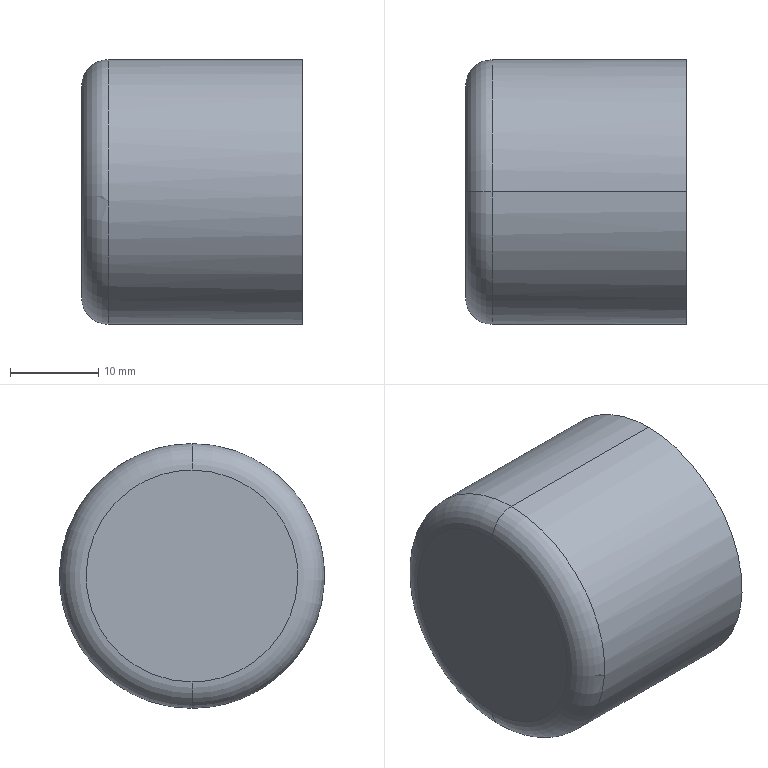Part | SolidWorks | features BaseBody 1 | 1 solid | 11 faces | box 25 x 30 x 30 mm | volume 13143 mm3 | cylinder 4 | plane 3 | cone 2 | torus 2 | commonest cylinder face diameters 18 x2 30 x2
STEP:
#1=CARTESIAN_POINT('',(7.,0.,6.));
#2=VERTEX_POINT('',#1);
#3=CARTESIAN_POINT('',(7.,0.,-6.));
#4=VERTEX_POINT('',#3);
#5=CARTESIAN_POINT('',(7.,0.,6.));
#6=CARTESIAN_POINT('',(7.,-0.7879,6.));
#7=CARTESIAN_POINT('',(7.,-1.568,5.845));
#8=CARTESIAN_POINT('',(7.,-3.024,5.242));
#9=CARTESIAN_POINT('',(7.,-3.685,4.8));
#10=CARTESIAN_POINT('',(7.,-4.8,3.685));
#11=CARTESIAN_POINT('',(7.,-5.242,3.024));
#12=CARTESIAN_POINT('',(7.,-5.845,1.568));
#13=CARTESIAN_POINT('',(7.,-6.,0.7879));
#14=CARTESIAN_POINT('',(7.,-6.,-0.7879));
#15=CARTESIAN_POINT('',(7.,-5.845,-1.568));
#16=CARTESIAN_POINT('',(7.,-5.242,-3.024));
#17=CARTESIAN_POINT('',(7.,-4.8,-3.685));
#18=CARTESIAN_POINT('',(7.,-3.685,-4.8));
#19=CARTESIAN_POINT('',(7.,-3.024,-5.242));
#20=CARTESIAN_POINT('',(7.,-1.568,-5.845));
#21=CARTESIAN_POINT('',(7.,-0.7879,-6.));
#22=CARTESIAN_POINT('',(7.,0.,-6.));
#23=B_SPLINE_CURVE_WITH_KNOTS('',3,(#5,#6,#7,#8,#9,#10,#11,#12,#13,#14,#15,#16,#17,#18,#19,#20,#21,#22),.UNSPECIFIED.,.F.,.F.,(4,2,2,2,2,2,2,2,4),(3.142,3.534,3.927,4.32,4.712,5.105,5.498,5.89,6.283),.UNSPECIFIED.);
#24=EDGE_CURVE('',#2,#4,#23,.T.);
#25=ORIENTED_EDGE('',*,*,#24,.F.);
#26=CARTESIAN_POINT('',(10.,0.,9.));
#27=VERTEX_POINT('',#26);
#28=CARTESIAN_POINT('',(10.,0.,9.));
#29=DIRECTION('',(0.7071,0.,0.7071));
#30=VECTOR('',#29,1000.);
#31=LINE('',#28,#30);
#32=EDGE_CURVE('',#2,#27,#31,.T.);
#33=ORIENTED_EDGE('',*,*,#32,.T.);
#34=CARTESIAN_POINT('',(10.,0.,-9.));
#35=VERTEX_POINT('',#34);
#36=CARTESIAN_POINT('',(10.,0.,9.));
#37=CARTESIAN_POINT('',(10.,-1.178,9.));
#38=CARTESIAN_POINT('',(10.,-2.356,8.766));
#39=CARTESIAN_POINT('',(10.,-4.533,7.864));
#40=CARTESIAN_POINT('',(10.,-5.531,7.197));
#41=CARTESIAN_POINT('',(10.,-7.197,5.531));
#42=CARTESIAN_POINT('',(10.,-7.864,4.533));
#43=CARTESIAN_POINT('',(10.,-8.766,2.356));
#44=CARTESIAN_POINT('',(10.,-9.,1.178));
#45=CARTESIAN_POINT('',(10.,-9.,-1.178));
#46=CARTESIAN_POINT('',(10.,-8.766,-2.356));
#47=CARTESIAN_POINT('',(10.,-7.864,-4.533));
#48=CARTESIAN_POINT('',(10.,-7.197,-5.531));
#49=CARTESIAN_POINT('',(10.,-5.531,-7.197));
#50=CARTESIAN_POINT('',(10.,-4.533,-7.864));
#51=CARTESIAN_POINT('',(10.,-2.356,-8.766));
#52=CARTESIAN_POINT('',(10.,-1.178,-9.));
#53=CARTESIAN_POINT('',(10.,0.,-9.));
#54=B_SPLINE_CURVE_WITH_KNOTS('',3,(#36,#37,#38,#39,#40,#41,#42,#43,#44,#45,#46,#47,#48,#49,#50,#51,#52,#53),.UNSPECIFIED.,.F.,.F.,(4,2,2,2,2,2,2,2,4),(3.142,3.534,3.927,4.32,4.712,5.105,5.498,5.89,6.283),.UNSPECIFIED.);
#55=EDGE_CURVE('',#27,#35,#54,.T.);
#56=ORIENTED_EDGE('',*,*,#55,.T.);
#57=CARTESIAN_POINT('',(10.,0.,-9.));
#58=DIRECTION('',(0.7071,0.,-0.7071));
#59=VECTOR('',#58,1000.);
#60=LINE('',#57,#59);
#61=EDGE_CURVE('',#4,#35,#60,.T.);
#62=ORIENTED_EDGE('',*,*,#61,.F.);
#63=EDGE_LOOP('',(#25,#33,#56,#62));
#64=FACE_OUTER_BOUND('',#63,.T.);
#65=CARTESIAN_POINT('',(10.,0.,0.));
#66=DIRECTION('',(1.,0.,0.));
#67=DIRECTION('',(0.,0.,-1.));
#68=AXIS2_PLACEMENT_3D('',#65,#66,#67);
#69=CONICAL_SURFACE('',#68,9.,0.7854);
#70=ADVANCED_FACE('',(#64),#69,.F.);
#71=ORIENTED_EDGE('',*,*,#55,.F.);
#72=CARTESIAN_POINT('',(25.,0.,9.));
#73=VERTEX_POINT('',#72);
#74=CARTESIAN_POINT('',(35.,0.,9.));
#75=DIRECTION('',(1.,0.,0.));
#76=VECTOR('',#75,1000.);
#77=LINE('',#74,#76);
#78=EDGE_CURVE('',#27,#73,#77,.T.);
#79=ORIENTED_EDGE('',*,*,#78,.T.);
#80=CARTESIAN_POINT('',(25.,0.,-9.));
#81=VERTEX_POINT('',#80);
#82=CARTESIAN_POINT('',(25.,0.,9.));
#83=CARTESIAN_POINT('',(25.,-1.178,9.));
#84=CARTESIAN_POINT('',(25.,-2.356,8.766));
#85=CARTESIAN_POINT('',(25.,-4.533,7.864));
#86=CARTESIAN_POINT('',(25.,-5.531,7.197));
#87=CARTESIAN_POINT('',(25.,-7.197,5.531));
#88=CARTESIAN_POINT('',(25.,-7.864,4.533));
#89=CARTESIAN_POINT('',(25.,-8.766,2.356));
#90=CARTESIAN_POINT('',(25.,-9.,1.178));
#91=CARTESIAN_POINT('',(25.,-9.,-1.178));
#92=CARTESIAN_POINT('',(25.,-8.766,-2.356));
#93=CARTESIAN_POINT('',(25.,-7.864,-4.533));
#94=CARTESIAN_POINT('',(25.,-7.197,-5.531));
#95=CARTESIAN_POINT('',(25.,-5.531,-7.197));
#96=CARTESIAN_POINT('',(25.,-4.533,-7.864));
#97=CARTESIAN_POINT('',(25.,-2.356,-8.766));
#98=CARTESIAN_POINT('',(25.,-1.178,-9.));
#99=CARTESIAN_POINT('',(25.,0.,-9.));
#100=B_SPLINE_CURVE_WITH_KNOTS('',3,(#82,#83,#84,#85,#86,#87,#88,#89,#90,#91,#92,#93,#94,#95,#96,#97,#98,#99),.UNSPECIFIED.,.F.,.F.,(4,2,2,2,2,2,2,2,4),(3.142,3.534,3.927,4.32,4.712,5.105,5.498,5.89,6.283),.UNSPECIFIED.);
#101=EDGE_CURVE('',#73,#81,#100,.T.);
#102=ORIENTED_EDGE('',*,*,#101,.T.);
#103=CARTESIAN_POINT('',(35.,0.,-9.));
#104=DIRECTION('',(1.,0.,0.));
#105=VECTOR('',#104,1000.);
#106=LINE('',#103,#105);
#107=EDGE_CURVE('',#35,#81,#106,.T.);
#108=ORIENTED_EDGE('',*,*,#107,.F.);
#109=EDGE_LOOP('',(#71,#79,#102,#108));
#110=FACE_OUTER_BOUND('',#109,.T.);
#111=CARTESIAN_POINT('',(35.,0.,0.));
#112=DIRECTION('',(1.,0.,0.));
#113=DIRECTION('',(0.,0.,-1.));
#114=AXIS2_PLACEMENT_3D('',#111,#112,#113);
#115=CYLINDRICAL_SURFACE('',#114,9.);
#116=ADVANCED_FACE('',(#110),#115,.F.);
#117=CARTESIAN_POINT('',(3.,0.,-15.));
#118=VERTEX_POINT('',#117);
#119=CARTESIAN_POINT('',(3.,0.,15.));
#120=VERTEX_POINT('',#119);
#121=CARTESIAN_POINT('',(3.,0.,-15.));
#122=CARTESIAN_POINT('',(3.,1.963,-15.));
#123=CARTESIAN_POINT('',(3.,3.926,-14.61));
#124=CARTESIAN_POINT('',(3.,7.554,-13.107));
#125=CARTESIAN_POINT('',(3.,9.218,-11.995));
#126=CARTESIAN_POINT('',(3.,11.995,-9.218));
#127=CARTESIAN_POINT('',(3.,13.107,-7.554));
#128=CARTESIAN_POINT('',(3.,14.61,-3.926));
#129=CARTESIAN_POINT('',(3.,15.,-1.963));
#130=CARTESIAN_POINT('',(3.,15.,1.963));
#131=CARTESIAN_POINT('',(3.,14.61,3.926));
#132=CARTESIAN_POINT('',(3.,13.107,7.554));
#133=CARTESIAN_POINT('',(3.,11.995,9.218));
#134=CARTESIAN_POINT('',(3.,9.218,11.995));
#135=CARTESIAN_POINT('',(3.,7.554,13.107));
#136=CARTESIAN_POINT('',(3.,3.926,14.61));
#137=CARTESIAN_POINT('',(3.,1.963,15.));
#138=CARTESIAN_POINT('',(3.,0.,15.));
#139=B_SPLINE_CURVE_WITH_KNOTS('',3,(#121,#122,#123,#124,#125,#126,#127,#128,#129,#130,#131,#132,#133,#134,#135,#136,#137,#138),.UNSPECIFIED.,.F.,.F.,(4,2,2,2,2,2,2,2,4),(0.,0.3927,0.7854,1.178,1.571,1.963,2.356,2.749,3.142),.UNSPECIFIED.);
#140=EDGE_CURVE('',#118,#120,#139,.T.);
#141=ORIENTED_EDGE('',*,*,#140,.T.);
#142=CARTESIAN_POINT('',(25.,0.,15.));
#143=VERTEX_POINT('',#142);
#144=CARTESIAN_POINT('',(35.,0.,15.));
#145=DIRECTION('',(1.,0.,0.));
#146=VECTOR('',#145,1000.);
#147=LINE('',#144,#146);
#148=EDGE_CURVE('',#120,#143,#147,.T.);
#149=ORIENTED_EDGE('',*,*,#148,.T.);
#150=CARTESIAN_POINT('',(25.,0.,-15.));
#151=VERTEX_POINT('',#150);
#152=CARTESIAN_POINT('',(25.,0.,-15.));
#153=CARTESIAN_POINT('',(25.,0.9849,-15.));
#154=CARTESIAN_POINT('',(25.,1.96,-14.904));
#155=CARTESIAN_POINT('',(25.,3.892,-14.52));
#156=CARTESIAN_POINT('',(25.,4.83,-14.235));
#157=CARTESIAN_POINT('',(25.,6.65,-13.481));
#158=CARTESIAN_POINT('',(25.,7.515,-13.019));
#159=CARTESIAN_POINT('',(25.,9.152,-11.925));
#160=CARTESIAN_POINT('',(25.,9.91,-11.303));
#161=CARTESIAN_POINT('',(25.,11.303,-9.91));
#162=CARTESIAN_POINT('',(25.,11.925,-9.152));
#163=CARTESIAN_POINT('',(25.,13.019,-7.515));
#164=CARTESIAN_POINT('',(25.,13.481,-6.65));
#165=CARTESIAN_POINT('',(25.,14.235,-4.83));
#166=CARTESIAN_POINT('',(25.,14.52,-3.892));
#167=CARTESIAN_POINT('',(25.,14.904,-1.96));
#168=CARTESIAN_POINT('',(25.,15.,-0.9849));
#169=CARTESIAN_POINT('',(25.,15.,0.9849));
#170=CARTESIAN_POINT('',(25.,14.904,1.96));
#171=CARTESIAN_POINT('',(25.,14.52,3.892));
#172=CARTESIAN_POINT('',(25.,14.235,4.83));
#173=CARTESIAN_POINT('',(25.,13.481,6.65));
#174=CARTESIAN_POINT('',(25.,13.019,7.515));
#175=CARTESIAN_POINT('',(25.,11.925,9.152));
#176=CARTESIAN_POINT('',(25.,11.303,9.91));
#177=CARTESIAN_POINT('',(25.,9.91,11.303));
#178=CARTESIAN_POINT('',(25.,9.152,11.925));
#179=CARTESIAN_POINT('',(25.,7.515,13.019));
#180=CARTESIAN_POINT('',(25.,6.65,13.481));
#181=CARTESIAN_POINT('',(25.,4.83,14.235));
#182=CARTESIAN_POINT('',(25.,3.892,14.52));
#183=CARTESIAN_POINT('',(25.,1.96,14.904));
#184=CARTESIAN_POINT('',(25.,0.9849,15.));
#185=CARTESIAN_POINT('',(25.,0.,15.));
#186=B_SPLINE_CURVE_WITH_KNOTS('',3,(#152,#153,#154,#155,#156,#157,#158,#159,#160,#161,#162,#163,#164,#165,#166,#167,#168,#169,#170,#171,#172,#173,#174,#175,#176,#177,#178,#179,#180,#181,#182,#183,#184,#185),.UNSPECIFIED.,.F.,.F.,(4,2,2,2,2,2,2,2,2,2,2,2,2,2,2,2,4),(0.,0.1963,0.3927,0.589,0.7854,0.9817,1.178,1.374,1.571,1.767,1.963,2.16,2.356,2.553,2.749,2.945,3.142),.UNSPECIFIED.);
#187=EDGE_CURVE('',#151,#143,#186,.T.);
#188=ORIENTED_EDGE('',*,*,#187,.F.);
#189=CARTESIAN_POINT('',(35.,0.,-15.));
#190=DIRECTION('',(1.,0.,0.));
#191=VECTOR('',#190,1000.);
#192=LINE('',#189,#191);
#193=EDGE_CURVE('',#118,#151,#192,.T.);
#194=ORIENTED_EDGE('',*,*,#193,.F.);
#195=EDGE_LOOP('',(#141,#149,#188,#194));
#196=FACE_OUTER_BOUND('',#195,.T.);
#197=CARTESIAN_POINT('',(35.,0.,0.));
#198=DIRECTION('',(1.,0.,0.));
#199=DIRECTION('',(0.,0.,-1.));
#200=AXIS2_PLACEMENT_3D('',#197,#198,#199);
#201=CYLINDRICAL_SURFACE('',#200,15.);
#202=ADVANCED_FACE('',(#196),#201,.T.);
#203=CARTESIAN_POINT('',(0.,0.,-12.));
#204=VERTEX_POINT('',#203);
#205=CARTESIAN_POINT('',(0.,0.,12.));
#206=VERTEX_POINT('',#205);
#207=CARTESIAN_POINT('',(0.,0.,-12.));
#208=CARTESIAN_POINT('',(0.,1.571,-12.));
#209=CARTESIAN_POINT('',(0.,3.141,-11.688));
#210=CARTESIAN_POINT('',(0.,6.043,-10.485));
#211=CARTESIAN_POINT('',(0.,7.375,-9.596));
#212=CARTESIAN_POINT('',(0.,9.596,-7.375));
#213=CARTESIAN_POINT('',(0.,10.485,-6.043));
#214=CARTESIAN_POINT('',(0.,11.688,-3.141));
#215=CARTESIAN_POINT('',(0.,12.,-1.571));
#216=CARTESIAN_POINT('',(0.,12.,1.571));
#217=CARTESIAN_POINT('',(0.,11.688,3.141));
#218=CARTESIAN_POINT('',(0.,10.485,6.043));
#219=CARTESIAN_POINT('',(0.,9.596,7.375));
#220=CARTESIAN_POINT('',(0.,7.375,9.596));
#221=CARTESIAN_POINT('',(0.,6.043,10.485));
#222=CARTESIAN_POINT('',(0.,3.141,11.688));
#223=CARTESIAN_POINT('',(0.,1.571,12.));
#224=CARTESIAN_POINT('',(0.,0.,12.));
#225=B_SPLINE_CURVE_WITH_KNOTS('',3,(#207,#208,#209,#210,#211,#212,#213,#214,#215,#216,#217,#218,#219,#220,#221,#222,#223,#224),.UNSPECIFIED.,.F.,.F.,(4,2,2,2,2,2,2,2,4),(0.,0.3927,0.7854,1.178,1.571,1.963,2.356,2.749,3.142),.UNSPECIFIED.);
#226=EDGE_CURVE('',#204,#206,#225,.T.);
#227=ORIENTED_EDGE('',*,*,#226,.T.);
#228=CARTESIAN_POINT('',(3.,0.,12.));
#229=DIRECTION('',(0.,1.,0.));
#230=DIRECTION('',(0.,0.,1.));
#231=AXIS2_PLACEMENT_3D('',#228,#229,#230);
#232=CIRCLE('',#231,3.);
#233=EDGE_CURVE('',#206,#120,#232,.T.);
#234=ORIENTED_EDGE('',*,*,#233,.T.);
#235=ORIENTED_EDGE('',*,*,#140,.F.);
#236=CARTESIAN_POINT('',(3.,0.,-12.));
#237=DIRECTION('',(0.,-1.,0.));
#238=DIRECTION('',(0.,0.,-1.));
#239=AXIS2_PLACEMENT_3D('',#236,#237,#238);
#240=CIRCLE('',#239,3.);
#241=EDGE_CURVE('',#204,#118,#240,.T.);
#242=ORIENTED_EDGE('',*,*,#241,.F.);
#243=EDGE_LOOP('',(#227,#234,#235,#242));
#244=FACE_OUTER_BOUND('',#243,.T.);
#245=CARTESIAN_POINT('',(3.,0.,0.));
#246=DIRECTION('',(1.,0.,0.));
#247=DIRECTION('',(0.,0.,-1.));
#248=AXIS2_PLACEMENT_3D('',#245,#246,#247);
#249=TOROIDAL_SURFACE('',#248,12.,3.);
#250=ADVANCED_FACE('',(#244),#249,.T.);
#251=ORIENTED_EDGE('',*,*,#226,.F.);
#252=CARTESIAN_POINT('',(0.,0.,12.));
#253=CARTESIAN_POINT('',(0.,-1.571,12.));
#254=CARTESIAN_POINT('',(0.,-3.141,11.688));
#255=CARTESIAN_POINT('',(0.,-6.043,10.485));
#256=CARTESIAN_POINT('',(0.,-7.375,9.596));
#257=CARTESIAN_POINT('',(0.,-9.596,7.375));
#258=CARTESIAN_POINT('',(0.,-10.485,6.043));
#259=CARTESIAN_POINT('',(0.,-11.688,3.141));
#260=CARTESIAN_POINT('',(0.,-12.,1.571));
#261=CARTESIAN_POINT('',(0.,-12.,-1.571));
#262=CARTESIAN_POINT('',(0.,-11.688,-3.141));
#263=CARTESIAN_POINT('',(0.,-10.485,-6.043));
#264=CARTESIAN_POINT('',(0.,-9.596,-7.375));
#265=CARTESIAN_POINT('',(0.,-7.375,-9.596));
#266=CARTESIAN_POINT('',(0.,-6.043,-10.485));
#267=CARTESIAN_POINT('',(0.,-3.141,-11.688));
#268=CARTESIAN_POINT('',(0.,-1.571,-12.));
#269=CARTESIAN_POINT('',(0.,0.,-12.));
#270=B_SPLINE_CURVE_WITH_KNOTS('',3,(#252,#253,#254,#255,#256,#257,#258,#259,#260,#261,#262,#263,#264,#265,#266,#267,#268,#269),.UNSPECIFIED.,.F.,.F.,(4,2,2,2,2,2,2,2,4),(3.142,3.534,3.927,4.32,4.712,5.105,5.498,5.89,6.283),.UNSPECIFIED.);
#271=EDGE_CURVE('',#206,#204,#270,.T.);
#272=ORIENTED_EDGE('',*,*,#271,.F.);
#273=EDGE_LOOP('',(#251,#272));
#274=FACE_OUTER_BOUND('',#273,.T.);
#275=CARTESIAN_POINT('',(0.,0.,0.));
#276=DIRECTION('',(1.,0.,0.));
#277=DIRECTION('',(0.,0.,-1.));
#278=AXIS2_PLACEMENT_3D('',#275,#276,#277);
#279=PLANE('',#278);
#280=ADVANCED_FACE('',(#274),#279,.F.);
#281=ORIENTED_EDGE('',*,*,#233,.F.);
#282=ORIENTED_EDGE('',*,*,#271,.T.);
#283=ORIENTED_EDGE('',*,*,#241,.T.);
#284=CARTESIAN_POINT('',(3.,0.,15.));
#285=CARTESIAN_POINT('',(3.,-1.963,15.));
#286=CARTESIAN_POINT('',(3.,-3.926,14.61));
#287=CARTESIAN_POINT('',(3.,-7.554,13.107));
#288=CARTESIAN_POINT('',(3.,-9.218,11.995));
#289=CARTESIAN_POINT('',(3.,-11.995,9.218));
#290=CARTESIAN_POINT('',(3.,-13.107,7.554));
#291=CARTESIAN_POINT('',(3.,-14.61,3.926));
#292=CARTESIAN_POINT('',(3.,-15.,1.963));
#293=CARTESIAN_POINT('',(3.,-15.,-1.963));
#294=CARTESIAN_POINT('',(3.,-14.61,-3.926));
#295=CARTESIAN_POINT('',(3.,-13.107,-7.554));
#296=CARTESIAN_POINT('',(3.,-11.995,-9.218));
#297=CARTESIAN_POINT('',(3.,-9.218,-11.995));
#298=CARTESIAN_POINT('',(3.,-7.554,-13.107));
#299=CARTESIAN_POINT('',(3.,-3.926,-14.61));
#300=CARTESIAN_POINT('',(3.,-1.963,-15.));
#301=CARTESIAN_POINT('',(3.,0.,-15.));
#302=B_SPLINE_CURVE_WITH_KNOTS('',3,(#284,#285,#286,#287,#288,#289,#290,#291,#292,#293,#294,#295,#296,#297,#298,#299,#300,#301),.UNSPECIFIED.,.F.,.F.,(4,2,2,2,2,2,2,2,4),(3.142,3.534,3.927,4.32,4.712,5.105,5.498,5.89,6.283),.UNSPECIFIED.);
#303=EDGE_CURVE('',#120,#118,#302,.T.);
#304=ORIENTED_EDGE('',*,*,#303,.F.);
#305=EDGE_LOOP('',(#281,#282,#283,#304));
#306=FACE_OUTER_BOUND('',#305,.T.);
#307=CARTESIAN_POINT('',(3.,0.,0.));
#308=DIRECTION('',(1.,0.,0.));
#309=DIRECTION('',(0.,0.,-1.));
#310=AXIS2_PLACEMENT_3D('',#307,#308,#309);
#311=TOROIDAL_SURFACE('',#310,12.,3.);
#312=ADVANCED_FACE('',(#306),#311,.T.);
#313=ORIENTED_EDGE('',*,*,#148,.F.);
#314=ORIENTED_EDGE('',*,*,#303,.T.);
#315=ORIENTED_EDGE('',*,*,#193,.T.);
#316=CARTESIAN_POINT('',(25.,0.,15.));
#317=CARTESIAN_POINT('',(25.,-0.9849,15.));
#318=CARTESIAN_POINT('',(25.,-1.96,14.904));
#319=CARTESIAN_POINT('',(25.,-3.892,14.52));
#320=CARTESIAN_POINT('',(25.,-4.83,14.235));
#321=CARTESIAN_POINT('',(25.,-6.65,13.481));
#322=CARTESIAN_POINT('',(25.,-7.515,13.019));
#323=CARTESIAN_POINT('',(25.,-9.152,11.925));
#324=CARTESIAN_POINT('',(25.,-9.91,11.303));
#325=CARTESIAN_POINT('',(25.,-11.303,9.91));
#326=CARTESIAN_POINT('',(25.,-11.925,9.152));
#327=CARTESIAN_POINT('',(25.,-13.019,7.515));
#328=CARTESIAN_POINT('',(25.,-13.481,6.65));
#329=CARTESIAN_POINT('',(25.,-14.235,4.83));
#330=CARTESIAN_POINT('',(25.,-14.52,3.892));
#331=CARTESIAN_POINT('',(25.,-14.904,1.96));
#332=CARTESIAN_POINT('',(25.,-15.,0.9849));
#333=CARTESIAN_POINT('',(25.,-15.,-0.9849));
#334=CARTESIAN_POINT('',(25.,-14.904,-1.96));
#335=CARTESIAN_POINT('',(25.,-14.52,-3.892));
#336=CARTESIAN_POINT('',(25.,-14.235,-4.83));
#337=CARTESIAN_POINT('',(25.,-13.481,-6.65));
#338=CARTESIAN_POINT('',(25.,-13.019,-7.515));
#339=CARTESIAN_POINT('',(25.,-11.925,-9.152));
#340=CARTESIAN_POINT('',(25.,-11.303,-9.91));
#341=CARTESIAN_POINT('',(25.,-9.91,-11.303));
#342=CARTESIAN_POINT('',(25.,-9.152,-11.925));
#343=CARTESIAN_POINT('',(25.,-7.515,-13.019));
#344=CARTESIAN_POINT('',(25.,-6.65,-13.481));
#345=CARTESIAN_POINT('',(25.,-4.83,-14.235));
#346=CARTESIAN_POINT('',(25.,-3.892,-14.52));
#347=CARTESIAN_POINT('',(25.,-1.96,-14.904));
#348=CARTESIAN_POINT('',(25.,-0.9849,-15.));
#349=CARTESIAN_POINT('',(25.,0.,-15.));
#350=B_SPLINE_CURVE_WITH_KNOTS('',3,(#316,#317,#318,#319,#320,#321,#322,#323,#324,#325,#326,#327,#328,#329,#330,#331,#332,#333,#334,#335,#336,#337,#338,#339,#340,#341,#342,#343,#344,#345,#346,#347,#348,#349),.UNSPECIFIED.,.F.,.F.,(4,2,2,2,2,2,2,2,2,2,2,2,2,2,2,2,4),(3.142,3.338,3.534,3.731,3.927,4.123,4.32,4.516,4.712,4.909,5.105,5.301,5.498,5.694,5.89,6.087,6.283),.UNSPECIFIED.);
#351=EDGE_CURVE('',#143,#151,#350,.T.);
#352=ORIENTED_EDGE('',*,*,#351,.F.);
#353=EDGE_LOOP('',(#313,#314,#315,#352));
#354=FACE_OUTER_BOUND('',#353,.T.);
#355=CARTESIAN_POINT('',(35.,0.,0.));
#356=DIRECTION('',(1.,0.,0.));
#357=DIRECTION('',(0.,0.,-1.));
#358=AXIS2_PLACEMENT_3D('',#355,#356,#357);
#359=CYLINDRICAL_SURFACE('',#358,15.);
#360=ADVANCED_FACE('',(#354),#359,.T.);
#361=CARTESIAN_POINT('',(25.,0.,-9.));
#362=CARTESIAN_POINT('',(25.,1.178,-9.));
#363=CARTESIAN_POINT('',(25.,2.356,-8.766));
#364=CARTESIAN_POINT('',(25.,4.533,-7.864));
#365=CARTESIAN_POINT('',(25.,5.531,-7.197));
#366=CARTESIAN_POINT('',(25.,7.197,-5.531));
#367=CARTESIAN_POINT('',(25.,7.864,-4.533));
#368=CARTESIAN_POINT('',(25.,8.766,-2.356));
#369=CARTESIAN_POINT('',(25.,9.,-1.178));
#370=CARTESIAN_POINT('',(25.,9.,1.178));
#371=CARTESIAN_POINT('',(25.,8.766,2.356));
#372=CARTESIAN_POINT('',(25.,7.864,4.533));
#373=CARTESIAN_POINT('',(25.,7.197,5.531));
#374=CARTESIAN_POINT('',(25.,5.531,7.197));
#375=CARTESIAN_POINT('',(25.,4.533,7.864));
#376=CARTESIAN_POINT('',(25.,2.356,8.766));
#377=CARTESIAN_POINT('',(25.,1.178,9.));
#378=CARTESIAN_POINT('',(25.,0.,9.));
#379=B_SPLINE_CURVE_WITH_KNOTS('',3,(#361,#362,#363,#364,#365,#366,#367,#368,#369,#370,#371,#372,#373,#374,#375,#376,#377,#378),.UNSPECIFIED.,.F.,.F.,(4,2,2,2,2,2,2,2,4),(0.,0.3927,0.7854,1.178,1.571,1.963,2.356,2.749,3.142),.UNSPECIFIED.);
#380=EDGE_CURVE('',#81,#73,#379,.T.);
#381=ORIENTED_EDGE('',*,*,#380,.F.);
#382=ORIENTED_EDGE('',*,*,#101,.F.);
#383=EDGE_LOOP('',(#381,#382));
#384=FACE_BOUND('',#383,.T.);
#385=ORIENTED_EDGE('',*,*,#187,.T.);
#386=ORIENTED_EDGE('',*,*,#351,.T.);
#387=EDGE_LOOP('',(#385,#386));
#388=FACE_OUTER_BOUND('',#387,.T.);
#389=CARTESIAN_POINT('',(25.,15.,0.));
#390=DIRECTION('',(-1.,0.,0.));
#391=DIRECTION('',(0.,0.,1.));
#392=AXIS2_PLACEMENT_3D('',#389,#390,#391);
#393=PLANE('',#392);
#394=ADVANCED_FACE('',(#384,#388),#393,.F.);
#395=ORIENTED_EDGE('',*,*,#78,.F.);
#396=CARTESIAN_POINT('',(10.,0.,-9.));
#397=CARTESIAN_POINT('',(10.,1.178,-9.));
#398=CARTESIAN_POINT('',(10.,2.356,-8.766));
#399=CARTESIAN_POINT('',(10.,4.533,-7.864));
#400=CARTESIAN_POINT('',(10.,5.531,-7.197));
#401=CARTESIAN_POINT('',(10.,7.197,-5.531));
#402=CARTESIAN_POINT('',(10.,7.864,-4.533));
#403=CARTESIAN_POINT('',(10.,8.766,-2.356));
#404=CARTESIAN_POINT('',(10.,9.,-1.178));
#405=CARTESIAN_POINT('',(10.,9.,1.178));
#406=CARTESIAN_POINT('',(10.,8.766,2.356));
#407=CARTESIAN_POINT('',(10.,7.864,4.533));
#408=CARTESIAN_POINT('',(10.,7.197,5.531));
#409=CARTESIAN_POINT('',(10.,5.531,7.197));
#410=CARTESIAN_POINT('',(10.,4.533,7.864));
#411=CARTESIAN_POINT('',(10.,2.356,8.766));
#412=CARTESIAN_POINT('',(10.,1.178,9.));
#413=CARTESIAN_POINT('',(10.,0.,9.));
#414=B_SPLINE_CURVE_WITH_KNOTS('',3,(#396,#397,#398,#399,#400,#401,#402,#403,#404,#405,#406,#407,#408,#409,#410,#411,#412,#413),.UNSPECIFIED.,.F.,.F.,(4,2,2,2,2,2,2,2,4),(0.,0.3927,0.7854,1.178,1.571,1.963,2.356,2.749,3.142),.UNSPECIFIED.);
#415=EDGE_CURVE('',#35,#27,#414,.T.);
#416=ORIENTED_EDGE('',*,*,#415,.F.);
#417=ORIENTED_EDGE('',*,*,#107,.T.);
#418=ORIENTED_EDGE('',*,*,#380,.T.);
#419=EDGE_LOOP('',(#395,#416,#417,#418));
#420=FACE_OUTER_BOUND('',#419,.T.);
#421=CARTESIAN_POINT('',(35.,0.,0.));
#422=DIRECTION('',(1.,0.,0.));
#423=DIRECTION('',(0.,0.,-1.));
#424=AXIS2_PLACEMENT_3D('',#421,#422,#423);
#425=CYLINDRICAL_SURFACE('',#424,9.);
#426=ADVANCED_FACE('',(#420),#425,.F.);
#427=ORIENTED_EDGE('',*,*,#32,.F.);
#428=CARTESIAN_POINT('',(7.,0.,-6.));
#429=CARTESIAN_POINT('',(7.,0.7879,-6.));
#430=CARTESIAN_POINT('',(7.,1.568,-5.845));
#431=CARTESIAN_POINT('',(7.,3.024,-5.242));
#432=CARTESIAN_POINT('',(7.,3.685,-4.8));
#433=CARTESIAN_POINT('',(7.,4.8,-3.685));
#434=CARTESIAN_POINT('',(7.,5.242,-3.024));
#435=CARTESIAN_POINT('',(7.,5.845,-1.568));
#436=CARTESIAN_POINT('',(7.,6.,-0.7879));
#437=CARTESIAN_POINT('',(7.,6.,0.7879));
#438=CARTESIAN_POINT('',(7.,5.845,1.568));
#439=CARTESIAN_POINT('',(7.,5.242,3.024));
#440=CARTESIAN_POINT('',(7.,4.8,3.685));
#441=CARTESIAN_POINT('',(7.,3.685,4.8));
#442=CARTESIAN_POINT('',(7.,3.024,5.242));
#443=CARTESIAN_POINT('',(7.,1.568,5.845));
#444=CARTESIAN_POINT('',(7.,0.7879,6.));
#445=CARTESIAN_POINT('',(7.,0.,6.));
#446=B_SPLINE_CURVE_WITH_KNOTS('',3,(#428,#429,#430,#431,#432,#433,#434,#435,#436,#437,#438,#439,#440,#441,#442,#443,#444,#445),.UNSPECIFIED.,.F.,.F.,(4,2,2,2,2,2,2,2,4),(0.,0.3927,0.7854,1.178,1.571,1.963,2.356,2.749,3.142),.UNSPECIFIED.);
#447=EDGE_CURVE('',#4,#2,#446,.T.);
#448=ORIENTED_EDGE('',*,*,#447,.F.);
#449=ORIENTED_EDGE('',*,*,#61,.T.);
#450=ORIENTED_EDGE('',*,*,#415,.T.);
#451=EDGE_LOOP('',(#427,#448,#449,#450));
#452=FACE_OUTER_BOUND('',#451,.T.);
#453=CARTESIAN_POINT('',(10.,0.,0.));
#454=DIRECTION('',(1.,0.,0.));
#455=DIRECTION('',(0.,0.,-1.));
#456=AXIS2_PLACEMENT_3D('',#453,#454,#455);
#457=CONICAL_SURFACE('',#456,9.,0.7854);
#458=ADVANCED_FACE('',(#452),#457,.F.);
#459=ORIENTED_EDGE('',*,*,#447,.T.);
#460=ORIENTED_EDGE('',*,*,#24,.T.);
#461=EDGE_LOOP('',(#459,#460));
#462=FACE_OUTER_BOUND('',#461,.T.);
#463=CARTESIAN_POINT('',(7.,6.,0.));
#464=DIRECTION('',(-1.,0.,0.));
#465=DIRECTION('',(0.,0.,1.));
#466=AXIS2_PLACEMENT_3D('',#463,#464,#465);
#467=PLANE('',#466);
#468=ADVANCED_FACE('',(#462),#467,.F.);
#469=CLOSED_SHELL('',(#70,#116,#202,#250,#280,#312,#360,#394,#426,#458,#468));
#470=MANIFOLD_SOLID_BREP('',#469);
#471=CARTESIAN_POINT('',(0.,0.,0.));
#472=DIRECTION('',(0.,0.,1.));
#473=DIRECTION('',(1.,0.,0.));
#474=AXIS2_PLACEMENT_3D('',#471,#472,#473);
#475=(LENGTH_UNIT()NAMED_UNIT(*)SI_UNIT(.MILLI.,.METRE.));
#476=UNCERTAINTY_MEASURE_WITH_UNIT(LENGTH_MEASURE(0.00001),#475,'','');
#477=(NAMED_UNIT(*)PLANE_ANGLE_UNIT()SI_UNIT($,.RADIAN.));
#478=(NAMED_UNIT(*)SI_UNIT($,.STERADIAN.)SOLID_ANGLE_UNIT());
#479=(GEOMETRIC_REPRESENTATION_CONTEXT(3)GLOBAL_UNCERTAINTY_ASSIGNED_CONTEXT((#476))GLOBAL_UNIT_ASSIGNED_CONTEXT((#475,#477,#478))REPRESENTATION_CONTEXT('',''));
#480=ADVANCED_BREP_SHAPE_REPRESENTATION('',(#470,#474),#479);